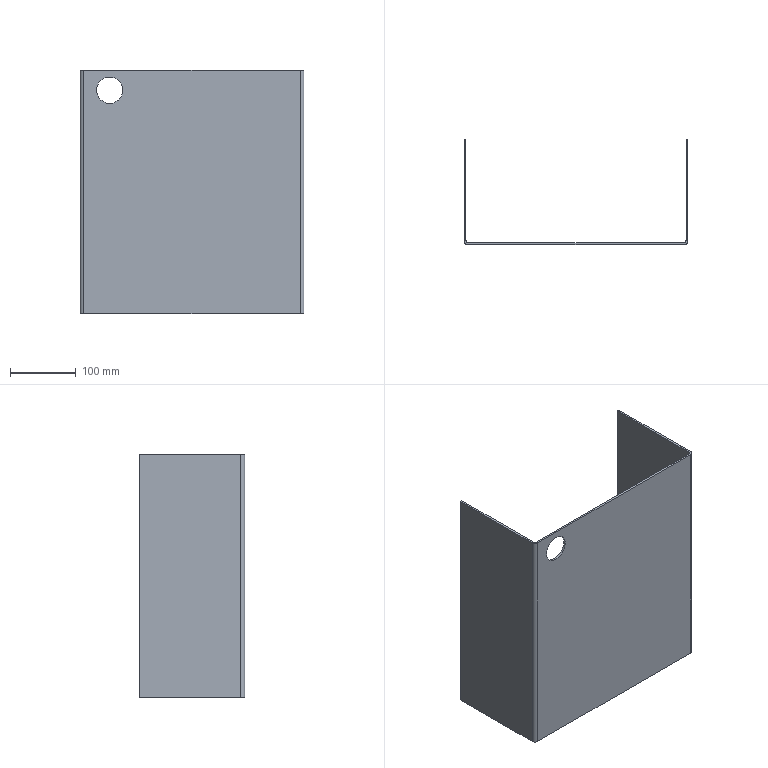Part | SolidWorks | features Cut 2, FlatPattern 1, SMBaseFlange 1, SheetMetal 1 | 1 solid | 26 faces | box 340 x 160 x 369 mm | volume 715620 mm3 | plane 18 | cylinder 8 | commonest cylinder face diameters 6 x2 11.5 x2 12 x2 40 x2
STEP:
#1=CARTESIAN_POINT('',(337.,145.,25.75));
#2=VERTEX_POINT('',#1);
#3=CARTESIAN_POINT('',(337.,145.,14.25));
#4=VERTEX_POINT('',#3);
#5=CARTESIAN_POINT('',(337.,145.,20.));
#6=DIRECTION('',(1.,0.,0.));
#7=DIRECTION('',(0.,0.,-1.));
#8=AXIS2_PLACEMENT_3D('',#5,#6,#7);
#9=CIRCLE('',#8,5.75);
#10=EDGE_CURVE('',#2,#4,#9,.T.);
#11=ORIENTED_EDGE('',*,*,#10,.F.);
#12=CARTESIAN_POINT('',(340.,145.,25.75));
#13=VERTEX_POINT('',#12);
#14=CARTESIAN_POINT('',(330.,145.,25.75));
#15=DIRECTION('',(1.,0.,0.));
#16=VECTOR('',#15,1000.);
#17=LINE('',#14,#16);
#18=EDGE_CURVE('',#2,#13,#17,.T.);
#19=ORIENTED_EDGE('',*,*,#18,.T.);
#20=CARTESIAN_POINT('',(340.,145.,14.25));
#21=VERTEX_POINT('',#20);
#22=CARTESIAN_POINT('',(340.,145.,20.));
#23=DIRECTION('',(1.,0.,0.));
#24=DIRECTION('',(0.,0.,-1.));
#25=AXIS2_PLACEMENT_3D('',#22,#23,#24);
#26=CIRCLE('',#25,5.75);
#27=EDGE_CURVE('',#13,#21,#26,.T.);
#28=ORIENTED_EDGE('',*,*,#27,.T.);
#29=CARTESIAN_POINT('',(330.,145.,14.25));
#30=DIRECTION('',(1.,0.,0.));
#31=VECTOR('',#30,1000.);
#32=LINE('',#29,#31);
#33=EDGE_CURVE('',#4,#21,#32,.T.);
#34=ORIENTED_EDGE('',*,*,#33,.F.);
#35=EDGE_LOOP('',(#11,#19,#28,#34));
#36=FACE_OUTER_BOUND('',#35,.T.);
#37=CARTESIAN_POINT('',(330.,145.,20.));
#38=DIRECTION('',(1.,0.,0.));
#39=DIRECTION('',(0.,0.,-1.));
#40=AXIS2_PLACEMENT_3D('',#37,#38,#39);
#41=CYLINDRICAL_SURFACE('',#40,5.75);
#42=ADVANCED_FACE('',(#36),#41,.F.);
#43=CARTESIAN_POINT('',(45.,3.,359.));
#44=VERTEX_POINT('',#43);
#45=CARTESIAN_POINT('',(45.,3.,319.));
#46=VERTEX_POINT('',#45);
#47=CARTESIAN_POINT('',(45.,3.,339.));
#48=DIRECTION('',(0.,-1.,0.));
#49=DIRECTION('',(0.,0.,-1.));
#50=AXIS2_PLACEMENT_3D('',#47,#48,#49);
#51=CIRCLE('',#50,20.);
#52=EDGE_CURVE('',#44,#46,#51,.T.);
#53=ORIENTED_EDGE('',*,*,#52,.F.);
#54=CARTESIAN_POINT('',(45.,0.,359.));
#55=VERTEX_POINT('',#54);
#56=CARTESIAN_POINT('',(45.,10.,359.));
#57=DIRECTION('',(0.,-1.,0.));
#58=VECTOR('',#57,1000.);
#59=LINE('',#56,#58);
#60=EDGE_CURVE('',#44,#55,#59,.T.);
#61=ORIENTED_EDGE('',*,*,#60,.T.);
#62=CARTESIAN_POINT('',(45.,0.,319.));
#63=VERTEX_POINT('',#62);
#64=CARTESIAN_POINT('',(45.,0.,339.));
#65=DIRECTION('',(0.,-1.,0.));
#66=DIRECTION('',(0.,0.,-1.));
#67=AXIS2_PLACEMENT_3D('',#64,#65,#66);
#68=CIRCLE('',#67,20.);
#69=EDGE_CURVE('',#55,#63,#68,.T.);
#70=ORIENTED_EDGE('',*,*,#69,.T.);
#71=CARTESIAN_POINT('',(45.,10.,319.));
#72=DIRECTION('',(0.,-1.,0.));
#73=VECTOR('',#72,1000.);
#74=LINE('',#71,#73);
#75=EDGE_CURVE('',#46,#63,#74,.T.);
#76=ORIENTED_EDGE('',*,*,#75,.F.);
#77=EDGE_LOOP('',(#53,#61,#70,#76));
#78=FACE_OUTER_BOUND('',#77,.T.);
#79=CARTESIAN_POINT('',(45.,10.,339.));
#80=DIRECTION('',(0.,-1.,0.));
#81=DIRECTION('',(0.,0.,-1.));
#82=AXIS2_PLACEMENT_3D('',#79,#80,#81);
#83=CYLINDRICAL_SURFACE('',#82,20.);
#84=ADVANCED_FACE('',(#78),#83,.F.);
#85=CARTESIAN_POINT('',(334.,0.,369.));
#86=VERTEX_POINT('',#85);
#87=CARTESIAN_POINT('',(334.,3.,369.));
#88=VERTEX_POINT('',#87);
#89=CARTESIAN_POINT('',(334.,0.,369.));
#90=DIRECTION('',(0.,1.,0.));
#91=VECTOR('',#90,1000.);
#92=LINE('',#89,#91);
#93=EDGE_CURVE('',#86,#88,#92,.T.);
#94=ORIENTED_EDGE('',*,*,#93,.F.);
#95=CARTESIAN_POINT('',(340.,6.,369.));
#96=VERTEX_POINT('',#95);
#97=CARTESIAN_POINT('',(334.,6.,369.));
#98=DIRECTION('',(0.,0.,-1.));
#99=DIRECTION('',(1.,0.,0.));
#100=AXIS2_PLACEMENT_3D('',#97,#98,#99);
#101=CIRCLE('',#100,6.);
#102=EDGE_CURVE('',#96,#86,#101,.T.);
#103=ORIENTED_EDGE('',*,*,#102,.F.);
#104=CARTESIAN_POINT('',(337.,6.,369.));
#105=VERTEX_POINT('',#104);
#106=CARTESIAN_POINT('',(337.,6.,369.));
#107=DIRECTION('',(1.,0.,0.));
#108=VECTOR('',#107,1000.);
#109=LINE('',#106,#108);
#110=EDGE_CURVE('',#105,#96,#109,.T.);
#111=ORIENTED_EDGE('',*,*,#110,.F.);
#112=CARTESIAN_POINT('',(334.,6.,369.));
#113=DIRECTION('',(0.,0.,-1.));
#114=DIRECTION('',(1.,0.,0.));
#115=AXIS2_PLACEMENT_3D('',#112,#113,#114);
#116=CIRCLE('',#115,3.);
#117=EDGE_CURVE('',#105,#88,#116,.T.);
#118=ORIENTED_EDGE('',*,*,#117,.T.);
#119=EDGE_LOOP('',(#94,#103,#111,#118));
#120=FACE_OUTER_BOUND('',#119,.T.);
#121=CARTESIAN_POINT('',(334.,0.,369.));
#122=DIRECTION('',(0.,0.,1.));
#123=DIRECTION('',(1.,0.,0.));
#124=AXIS2_PLACEMENT_3D('',#121,#122,#123);
#125=PLANE('',#124);
#126=ADVANCED_FACE('',(#120),#125,.T.);
#127=CARTESIAN_POINT('',(6.,0.,369.));
#128=VERTEX_POINT('',#127);
#129=CARTESIAN_POINT('',(0.,0.,369.));
#130=DIRECTION('',(-1.,0.,0.));
#131=VECTOR('',#130,1000.);
#132=LINE('',#129,#131);
#133=EDGE_CURVE('',#86,#128,#132,.T.);
#134=ORIENTED_EDGE('',*,*,#133,.F.);
#135=ORIENTED_EDGE('',*,*,#93,.T.);
#136=CARTESIAN_POINT('',(6.,3.,369.));
#137=VERTEX_POINT('',#136);
#138=CARTESIAN_POINT('',(0.,3.,369.));
#139=DIRECTION('',(-1.,0.,0.));
#140=VECTOR('',#139,1000.);
#141=LINE('',#138,#140);
#142=EDGE_CURVE('',#88,#137,#141,.T.);
#143=ORIENTED_EDGE('',*,*,#142,.T.);
#144=CARTESIAN_POINT('',(6.,3.,369.));
#145=DIRECTION('',(0.,-1.,0.));
#146=VECTOR('',#145,1000.);
#147=LINE('',#144,#146);
#148=EDGE_CURVE('',#137,#128,#147,.T.);
#149=ORIENTED_EDGE('',*,*,#148,.T.);
#150=EDGE_LOOP('',(#134,#135,#143,#149));
#151=FACE_OUTER_BOUND('',#150,.T.);
#152=CARTESIAN_POINT('',(337.,6.,369.));
#153=DIRECTION('',(0.,0.,1.));
#154=DIRECTION('',(1.,0.,0.));
#155=AXIS2_PLACEMENT_3D('',#152,#153,#154);
#156=PLANE('',#155);
#157=ADVANCED_FACE('',(#151),#156,.T.);
#158=CARTESIAN_POINT('',(340.,6.,0.));
#159=VERTEX_POINT('',#158);
#160=CARTESIAN_POINT('',(337.,6.,0.));
#161=VERTEX_POINT('',#160);
#162=CARTESIAN_POINT('',(340.,6.,0.));
#163=DIRECTION('',(-1.,0.,0.));
#164=VECTOR('',#163,1000.);
#165=LINE('',#162,#164);
#166=EDGE_CURVE('',#159,#161,#165,.T.);
#167=ORIENTED_EDGE('',*,*,#166,.F.);
#168=CARTESIAN_POINT('',(334.,0.,0.));
#169=VERTEX_POINT('',#168);
#170=CARTESIAN_POINT('',(334.,6.,0.));
#171=DIRECTION('',(0.,0.,-1.));
#172=DIRECTION('',(1.,0.,0.));
#173=AXIS2_PLACEMENT_3D('',#170,#171,#172);
#174=CIRCLE('',#173,6.);
#175=EDGE_CURVE('',#159,#169,#174,.T.);
#176=ORIENTED_EDGE('',*,*,#175,.T.);
#177=CARTESIAN_POINT('',(334.,3.,0.));
#178=VERTEX_POINT('',#177);
#179=CARTESIAN_POINT('',(334.,3.,0.));
#180=DIRECTION('',(0.,-1.,0.));
#181=VECTOR('',#180,1000.);
#182=LINE('',#179,#181);
#183=EDGE_CURVE('',#178,#169,#182,.T.);
#184=ORIENTED_EDGE('',*,*,#183,.F.);
#185=CARTESIAN_POINT('',(334.,6.,0.));
#186=DIRECTION('',(0.,0.,-1.));
#187=DIRECTION('',(1.,0.,0.));
#188=AXIS2_PLACEMENT_3D('',#185,#186,#187);
#189=CIRCLE('',#188,3.);
#190=EDGE_CURVE('',#161,#178,#189,.T.);
#191=ORIENTED_EDGE('',*,*,#190,.F.);
#192=EDGE_LOOP('',(#167,#176,#184,#191));
#193=FACE_OUTER_BOUND('',#192,.T.);
#194=CARTESIAN_POINT('',(340.,6.,0.));
#195=DIRECTION('',(0.,0.,-1.));
#196=DIRECTION('',(-1.,0.,0.));
#197=AXIS2_PLACEMENT_3D('',#194,#195,#196);
#198=PLANE('',#197);
#199=ADVANCED_FACE('',(#193),#198,.T.);
#200=CARTESIAN_POINT('',(340.,160.,0.));
#201=VERTEX_POINT('',#200);
#202=CARTESIAN_POINT('',(340.,0.,0.));
#203=DIRECTION('',(0.,-1.,0.));
#204=VECTOR('',#203,1000.);
#205=LINE('',#202,#204);
#206=EDGE_CURVE('',#201,#159,#205,.T.);
#207=ORIENTED_EDGE('',*,*,#206,.T.);
#208=ORIENTED_EDGE('',*,*,#166,.T.);
#209=CARTESIAN_POINT('',(337.,160.,0.));
#210=VERTEX_POINT('',#209);
#211=CARTESIAN_POINT('',(337.,0.,0.));
#212=DIRECTION('',(0.,-1.,0.));
#213=VECTOR('',#212,1000.);
#214=LINE('',#211,#213);
#215=EDGE_CURVE('',#210,#161,#214,.T.);
#216=ORIENTED_EDGE('',*,*,#215,.F.);
#217=CARTESIAN_POINT('',(337.,160.,0.));
#218=DIRECTION('',(1.,0.,0.));
#219=VECTOR('',#218,1000.);
#220=LINE('',#217,#219);
#221=EDGE_CURVE('',#210,#201,#220,.T.);
#222=ORIENTED_EDGE('',*,*,#221,.T.);
#223=EDGE_LOOP('',(#207,#208,#216,#222));
#224=FACE_OUTER_BOUND('',#223,.T.);
#225=CARTESIAN_POINT('',(334.,3.,0.));
#226=DIRECTION('',(0.,0.,-1.));
#227=DIRECTION('',(-1.,0.,0.));
#228=AXIS2_PLACEMENT_3D('',#225,#226,#227);
#229=PLANE('',#228);
#230=ADVANCED_FACE('',(#224),#229,.T.);
#231=CARTESIAN_POINT('',(0.,6.,369.));
#232=VERTEX_POINT('',#231);
#233=CARTESIAN_POINT('',(3.,6.,369.));
#234=VERTEX_POINT('',#233);
#235=CARTESIAN_POINT('',(0.,6.,369.));
#236=DIRECTION('',(1.,0.,0.));
#237=VECTOR('',#236,1000.);
#238=LINE('',#235,#237);
#239=EDGE_CURVE('',#232,#234,#238,.T.);
#240=ORIENTED_EDGE('',*,*,#239,.F.);
#241=CARTESIAN_POINT('',(6.,6.,369.));
#242=DIRECTION('',(0.,0.,-1.));
#243=DIRECTION('',(1.,0.,0.));
#244=AXIS2_PLACEMENT_3D('',#241,#242,#243);
#245=CIRCLE('',#244,6.);
#246=EDGE_CURVE('',#128,#232,#245,.T.);
#247=ORIENTED_EDGE('',*,*,#246,.F.);
#248=ORIENTED_EDGE('',*,*,#148,.F.);
#249=CARTESIAN_POINT('',(6.,6.,369.));
#250=DIRECTION('',(0.,0.,-1.));
#251=DIRECTION('',(1.,0.,0.));
#252=AXIS2_PLACEMENT_3D('',#249,#250,#251);
#253=CIRCLE('',#252,3.);
#254=EDGE_CURVE('',#137,#234,#253,.T.);
#255=ORIENTED_EDGE('',*,*,#254,.T.);
#256=EDGE_LOOP('',(#240,#247,#248,#255));
#257=FACE_OUTER_BOUND('',#256,.T.);
#258=CARTESIAN_POINT('',(0.,6.,369.));
#259=DIRECTION('',(0.,0.,1.));
#260=DIRECTION('',(1.,0.,0.));
#261=AXIS2_PLACEMENT_3D('',#258,#259,#260);
#262=PLANE('',#261);
#263=ADVANCED_FACE('',(#257),#262,.T.);
#264=CARTESIAN_POINT('',(0.,160.,369.));
#265=VERTEX_POINT('',#264);
#266=CARTESIAN_POINT('',(0.,0.,369.));
#267=DIRECTION('',(0.,1.,0.));
#268=VECTOR('',#267,1000.);
#269=LINE('',#266,#268);
#270=EDGE_CURVE('',#232,#265,#269,.T.);
#271=ORIENTED_EDGE('',*,*,#270,.F.);
#272=ORIENTED_EDGE('',*,*,#239,.T.);
#273=CARTESIAN_POINT('',(3.,160.,369.));
#274=VERTEX_POINT('',#273);
#275=CARTESIAN_POINT('',(3.,0.,369.));
#276=DIRECTION('',(0.,1.,0.));
#277=VECTOR('',#276,1000.);
#278=LINE('',#275,#277);
#279=EDGE_CURVE('',#234,#274,#278,.T.);
#280=ORIENTED_EDGE('',*,*,#279,.T.);
#281=CARTESIAN_POINT('',(0.,160.,369.));
#282=DIRECTION('',(1.,0.,0.));
#283=VECTOR('',#282,1000.);
#284=LINE('',#281,#283);
#285=EDGE_CURVE('',#265,#274,#284,.T.);
#286=ORIENTED_EDGE('',*,*,#285,.F.);
#287=EDGE_LOOP('',(#271,#272,#280,#286));
#288=FACE_OUTER_BOUND('',#287,.T.);
#289=CARTESIAN_POINT('',(6.,3.,369.));
#290=DIRECTION('',(0.,0.,1.));
#291=DIRECTION('',(1.,0.,0.));
#292=AXIS2_PLACEMENT_3D('',#289,#290,#291);
#293=PLANE('',#292);
#294=ADVANCED_FACE('',(#288),#293,.T.);
#295=CARTESIAN_POINT('',(6.,0.,0.));
#296=VERTEX_POINT('',#295);
#297=CARTESIAN_POINT('',(6.,3.,0.));
#298=VERTEX_POINT('',#297);
#299=CARTESIAN_POINT('',(6.,0.,0.));
#300=DIRECTION('',(0.,1.,0.));
#301=VECTOR('',#300,1000.);
#302=LINE('',#299,#301);
#303=EDGE_CURVE('',#296,#298,#302,.T.);
#304=ORIENTED_EDGE('',*,*,#303,.F.);
#305=CARTESIAN_POINT('',(0.,6.,0.));
#306=VERTEX_POINT('',#305);
#307=CARTESIAN_POINT('',(6.,6.,0.));
#308=DIRECTION('',(0.,0.,-1.));
#309=DIRECTION('',(1.,0.,0.));
#310=AXIS2_PLACEMENT_3D('',#307,#308,#309);
#311=CIRCLE('',#310,6.);
#312=EDGE_CURVE('',#296,#306,#311,.T.);
#313=ORIENTED_EDGE('',*,*,#312,.T.);
#314=CARTESIAN_POINT('',(3.,6.,0.));
#315=VERTEX_POINT('',#314);
#316=CARTESIAN_POINT('',(3.,6.,0.));
#317=DIRECTION('',(-1.,0.,0.));
#318=VECTOR('',#317,1000.);
#319=LINE('',#316,#318);
#320=EDGE_CURVE('',#315,#306,#319,.T.);
#321=ORIENTED_EDGE('',*,*,#320,.F.);
#322=CARTESIAN_POINT('',(6.,6.,0.));
#323=DIRECTION('',(0.,0.,-1.));
#324=DIRECTION('',(1.,0.,0.));
#325=AXIS2_PLACEMENT_3D('',#322,#323,#324);
#326=CIRCLE('',#325,3.);
#327=EDGE_CURVE('',#298,#315,#326,.T.);
#328=ORIENTED_EDGE('',*,*,#327,.F.);
#329=EDGE_LOOP('',(#304,#313,#321,#328));
#330=FACE_OUTER_BOUND('',#329,.T.);
#331=CARTESIAN_POINT('',(6.,0.,0.));
#332=DIRECTION('',(0.,0.,-1.));
#333=DIRECTION('',(-1.,0.,0.));
#334=AXIS2_PLACEMENT_3D('',#331,#332,#333);
#335=PLANE('',#334);
#336=ADVANCED_FACE('',(#330),#335,.T.);
#337=CARTESIAN_POINT('',(0.,0.,0.));
#338=DIRECTION('',(-1.,0.,0.));
#339=VECTOR('',#338,1000.);
#340=LINE('',#337,#339);
#341=EDGE_CURVE('',#169,#296,#340,.T.);
#342=ORIENTED_EDGE('',*,*,#341,.T.);
#343=ORIENTED_EDGE('',*,*,#303,.T.);
#344=CARTESIAN_POINT('',(0.,3.,0.));
#345=DIRECTION('',(-1.,0.,0.));
#346=VECTOR('',#345,1000.);
#347=LINE('',#344,#346);
#348=EDGE_CURVE('',#178,#298,#347,.T.);
#349=ORIENTED_EDGE('',*,*,#348,.F.);
#350=ORIENTED_EDGE('',*,*,#183,.T.);
#351=EDGE_LOOP('',(#342,#343,#349,#350));
#352=FACE_OUTER_BOUND('',#351,.T.);
#353=CARTESIAN_POINT('',(3.,6.,0.));
#354=DIRECTION('',(0.,0.,-1.));
#355=DIRECTION('',(-1.,0.,0.));
#356=AXIS2_PLACEMENT_3D('',#353,#354,#355);
#357=PLANE('',#356);
#358=ADVANCED_FACE('',(#352),#357,.T.);
#359=CARTESIAN_POINT('',(3.,160.,0.));
#360=VERTEX_POINT('',#359);
#361=CARTESIAN_POINT('',(3.,0.,0.));
#362=DIRECTION('',(0.,1.,0.));
#363=VECTOR('',#362,1000.);
#364=LINE('',#361,#363);
#365=EDGE_CURVE('',#315,#360,#364,.T.);
#366=ORIENTED_EDGE('',*,*,#365,.T.);
#367=CARTESIAN_POINT('',(3.,160.,369.));
#368=DIRECTION('',(0.,0.,-1.));
#369=VECTOR('',#368,1000.);
#370=LINE('',#367,#369);
#371=EDGE_CURVE('',#274,#360,#370,.T.);
#372=ORIENTED_EDGE('',*,*,#371,.F.);
#373=ORIENTED_EDGE('',*,*,#279,.F.);
#374=CARTESIAN_POINT('',(3.,6.,369.));
#375=DIRECTION('',(0.,0.,-1.));
#376=VECTOR('',#375,1000.);
#377=LINE('',#374,#376);
#378=EDGE_CURVE('',#234,#315,#377,.T.);
#379=ORIENTED_EDGE('',*,*,#378,.T.);
#380=EDGE_LOOP('',(#366,#372,#373,#379));
#381=FACE_OUTER_BOUND('',#380,.T.);
#382=CARTESIAN_POINT('',(3.,0.,369.));
#383=DIRECTION('',(-1.,0.,0.));
#384=DIRECTION('',(0.,0.,1.));
#385=AXIS2_PLACEMENT_3D('',#382,#383,#384);
#386=PLANE('',#385);
#387=ADVANCED_FACE('',(#381),#386,.F.);
#388=CARTESIAN_POINT('',(0.,160.,0.));
#389=VERTEX_POINT('',#388);
#390=CARTESIAN_POINT('',(0.,160.,0.));
#391=DIRECTION('',(1.,0.,0.));
#392=VECTOR('',#391,1000.);
#393=LINE('',#390,#392);
#394=EDGE_CURVE('',#389,#360,#393,.T.);
#395=ORIENTED_EDGE('',*,*,#394,.F.);
#396=CARTESIAN_POINT('',(0.,160.,369.));
#397=DIRECTION('',(0.,0.,-1.));
#398=VECTOR('',#397,1000.);
#399=LINE('',#396,#398);
#400=EDGE_CURVE('',#265,#389,#399,.T.);
#401=ORIENTED_EDGE('',*,*,#400,.F.);
#402=ORIENTED_EDGE('',*,*,#285,.T.);
#403=ORIENTED_EDGE('',*,*,#371,.T.);
#404=EDGE_LOOP('',(#395,#401,#402,#403));
#405=FACE_OUTER_BOUND('',#404,.T.);
#406=CARTESIAN_POINT('',(0.,160.,369.));
#407=DIRECTION('',(0.,1.,0.));
#408=DIRECTION('',(0.,0.,1.));
#409=AXIS2_PLACEMENT_3D('',#406,#407,#408);
#410=PLANE('',#409);
#411=ADVANCED_FACE('',(#405),#410,.T.);
#412=CARTESIAN_POINT('',(0.,0.,0.));
#413=DIRECTION('',(0.,1.,0.));
#414=VECTOR('',#413,1000.);
#415=LINE('',#412,#414);
#416=EDGE_CURVE('',#306,#389,#415,.T.);
#417=ORIENTED_EDGE('',*,*,#416,.F.);
#418=CARTESIAN_POINT('',(0.,6.,369.));
#419=DIRECTION('',(0.,0.,-1.));
#420=VECTOR('',#419,1000.);
#421=LINE('',#418,#420);
#422=EDGE_CURVE('',#232,#306,#421,.T.);
#423=ORIENTED_EDGE('',*,*,#422,.F.);
#424=ORIENTED_EDGE('',*,*,#270,.T.);
#425=ORIENTED_EDGE('',*,*,#400,.T.);
#426=EDGE_LOOP('',(#417,#423,#424,#425));
#427=FACE_OUTER_BOUND('',#426,.T.);
#428=CARTESIAN_POINT('',(0.,0.,369.));
#429=DIRECTION('',(-1.,0.,0.));
#430=DIRECTION('',(0.,0.,1.));
#431=AXIS2_PLACEMENT_3D('',#428,#429,#430);
#432=PLANE('',#431);
#433=ADVANCED_FACE('',(#427),#432,.T.);
#434=ORIENTED_EDGE('',*,*,#312,.F.);
#435=CARTESIAN_POINT('',(6.,0.,369.));
#436=DIRECTION('',(0.,0.,-1.));
#437=VECTOR('',#436,1000.);
#438=LINE('',#435,#437);
#439=EDGE_CURVE('',#128,#296,#438,.T.);
#440=ORIENTED_EDGE('',*,*,#439,.F.);
#441=ORIENTED_EDGE('',*,*,#246,.T.);
#442=ORIENTED_EDGE('',*,*,#422,.T.);
#443=EDGE_LOOP('',(#434,#440,#441,#442));
#444=FACE_OUTER_BOUND('',#443,.T.);
#445=CARTESIAN_POINT('',(6.,6.,369.));
#446=DIRECTION('',(0.,0.,-1.));
#447=DIRECTION('',(-1.,0.,0.));
#448=AXIS2_PLACEMENT_3D('',#445,#446,#447);
#449=CYLINDRICAL_SURFACE('',#448,6.);
#450=ADVANCED_FACE('',(#444),#449,.T.);
#451=CARTESIAN_POINT('',(45.,0.,339.));
#452=DIRECTION('',(0.,-1.,0.));
#453=DIRECTION('',(0.,0.,-1.));
#454=AXIS2_PLACEMENT_3D('',#451,#452,#453);
#455=CIRCLE('',#454,20.);
#456=EDGE_CURVE('',#63,#55,#455,.T.);
#457=ORIENTED_EDGE('',*,*,#456,.F.);
#458=ORIENTED_EDGE('',*,*,#69,.F.);
#459=EDGE_LOOP('',(#457,#458));
#460=FACE_BOUND('',#459,.T.);
#461=ORIENTED_EDGE('',*,*,#341,.F.);
#462=CARTESIAN_POINT('',(334.,0.,369.));
#463=DIRECTION('',(0.,0.,-1.));
#464=VECTOR('',#463,1000.);
#465=LINE('',#462,#464);
#466=EDGE_CURVE('',#86,#169,#465,.T.);
#467=ORIENTED_EDGE('',*,*,#466,.F.);
#468=ORIENTED_EDGE('',*,*,#133,.T.);
#469=ORIENTED_EDGE('',*,*,#439,.T.);
#470=EDGE_LOOP('',(#461,#467,#468,#469));
#471=FACE_OUTER_BOUND('',#470,.T.);
#472=CARTESIAN_POINT('',(0.,0.,369.));
#473=DIRECTION('',(0.,-1.,0.));
#474=DIRECTION('',(0.,0.,-1.));
#475=AXIS2_PLACEMENT_3D('',#472,#473,#474);
#476=PLANE('',#475);
#477=ADVANCED_FACE('',(#460,#471),#476,.T.);
#478=ORIENTED_EDGE('',*,*,#175,.F.);
#479=CARTESIAN_POINT('',(340.,6.,369.));
#480=DIRECTION('',(0.,0.,-1.));
#481=VECTOR('',#480,1000.);
#482=LINE('',#479,#481);
#483=EDGE_CURVE('',#96,#159,#482,.T.);
#484=ORIENTED_EDGE('',*,*,#483,.F.);
#485=ORIENTED_EDGE('',*,*,#102,.T.);
#486=ORIENTED_EDGE('',*,*,#466,.T.);
#487=EDGE_LOOP('',(#478,#484,#485,#486));
#488=FACE_OUTER_BOUND('',#487,.T.);
#489=CARTESIAN_POINT('',(334.,6.,369.));
#490=DIRECTION('',(0.,0.,-1.));
#491=DIRECTION('',(-1.,0.,0.));
#492=AXIS2_PLACEMENT_3D('',#489,#490,#491);
#493=CYLINDRICAL_SURFACE('',#492,6.);
#494=ADVANCED_FACE('',(#488),#493,.T.);
#495=CARTESIAN_POINT('',(340.,145.,20.));
#496=DIRECTION('',(1.,0.,0.));
#497=DIRECTION('',(0.,0.,-1.));
#498=AXIS2_PLACEMENT_3D('',#495,#496,#497);
#499=CIRCLE('',#498,5.75);
#500=EDGE_CURVE('',#21,#13,#499,.T.);
#501=ORIENTED_EDGE('',*,*,#500,.F.);
#502=ORIENTED_EDGE('',*,*,#27,.F.);
#503=EDGE_LOOP('',(#501,#502));
#504=FACE_BOUND('',#503,.T.);
#505=ORIENTED_EDGE('',*,*,#206,.F.);
#506=CARTESIAN_POINT('',(340.,160.,369.));
#507=VERTEX_POINT('',#506);
#508=CARTESIAN_POINT('',(340.,160.,369.));
#509=DIRECTION('',(0.,0.,-1.));
#510=VECTOR('',#509,1000.);
#511=LINE('',#508,#510);
#512=EDGE_CURVE('',#507,#201,#511,.T.);
#513=ORIENTED_EDGE('',*,*,#512,.F.);
#514=CARTESIAN_POINT('',(340.,0.,369.));
#515=DIRECTION('',(0.,-1.,0.));
#516=VECTOR('',#515,1000.);
#517=LINE('',#514,#516);
#518=EDGE_CURVE('',#507,#96,#517,.T.);
#519=ORIENTED_EDGE('',*,*,#518,.T.);
#520=ORIENTED_EDGE('',*,*,#483,.T.);
#521=EDGE_LOOP('',(#505,#513,#519,#520));
#522=FACE_OUTER_BOUND('',#521,.T.);
#523=CARTESIAN_POINT('',(340.,0.,369.));
#524=DIRECTION('',(1.,0.,0.));
#525=DIRECTION('',(0.,0.,-1.));
#526=AXIS2_PLACEMENT_3D('',#523,#524,#525);
#527=PLANE('',#526);
#528=ADVANCED_FACE('',(#504,#522),#527,.T.);
#529=ORIENTED_EDGE('',*,*,#221,.F.);
#530=CARTESIAN_POINT('',(337.,160.,369.));
#531=VERTEX_POINT('',#530);
#532=CARTESIAN_POINT('',(337.,160.,369.));
#533=DIRECTION('',(0.,0.,-1.));
#534=VECTOR('',#533,1000.);
#535=LINE('',#532,#534);
#536=EDGE_CURVE('',#531,#210,#535,.T.);
#537=ORIENTED_EDGE('',*,*,#536,.F.);
#538=CARTESIAN_POINT('',(337.,160.,369.));
#539=DIRECTION('',(1.,0.,0.));
#540=VECTOR('',#539,1000.);
#541=LINE('',#538,#540);
#542=EDGE_CURVE('',#531,#507,#541,.T.);
#543=ORIENTED_EDGE('',*,*,#542,.T.);
#544=ORIENTED_EDGE('',*,*,#512,.T.);
#545=EDGE_LOOP('',(#529,#537,#543,#544));
#546=FACE_OUTER_BOUND('',#545,.T.);
#547=CARTESIAN_POINT('',(337.,160.,369.));
#548=DIRECTION('',(0.,1.,0.));
#549=DIRECTION('',(0.,0.,1.));
#550=AXIS2_PLACEMENT_3D('',#547,#548,#549);
#551=PLANE('',#550);
#552=ADVANCED_FACE('',(#546),#551,.T.);
#553=CARTESIAN_POINT('',(337.,145.,20.));
#554=DIRECTION('',(1.,0.,0.));
#555=DIRECTION('',(0.,0.,-1.));
#556=AXIS2_PLACEMENT_3D('',#553,#554,#555);
#557=CIRCLE('',#556,5.75);
#558=EDGE_CURVE('',#4,#2,#557,.T.);
#559=ORIENTED_EDGE('',*,*,#558,.T.);
#560=ORIENTED_EDGE('',*,*,#10,.T.);
#561=EDGE_LOOP('',(#559,#560));
#562=FACE_BOUND('',#561,.T.);
#563=ORIENTED_EDGE('',*,*,#215,.T.);
#564=CARTESIAN_POINT('',(337.,6.,369.));
#565=DIRECTION('',(0.,0.,-1.));
#566=VECTOR('',#565,1000.);
#567=LINE('',#564,#566);
#568=EDGE_CURVE('',#105,#161,#567,.T.);
#569=ORIENTED_EDGE('',*,*,#568,.F.);
#570=CARTESIAN_POINT('',(337.,0.,369.));
#571=DIRECTION('',(0.,-1.,0.));
#572=VECTOR('',#571,1000.);
#573=LINE('',#570,#572);
#574=EDGE_CURVE('',#531,#105,#573,.T.);
#575=ORIENTED_EDGE('',*,*,#574,.F.);
#576=ORIENTED_EDGE('',*,*,#536,.T.);
#577=EDGE_LOOP('',(#563,#569,#575,#576));
#578=FACE_OUTER_BOUND('',#577,.T.);
#579=CARTESIAN_POINT('',(337.,0.,369.));
#580=DIRECTION('',(1.,0.,0.));
#581=DIRECTION('',(0.,0.,-1.));
#582=AXIS2_PLACEMENT_3D('',#579,#580,#581);
#583=PLANE('',#582);
#584=ADVANCED_FACE('',(#562,#578),#583,.F.);
#585=ORIENTED_EDGE('',*,*,#190,.T.);
#586=CARTESIAN_POINT('',(334.,3.,369.));
#587=DIRECTION('',(0.,0.,-1.));
#588=VECTOR('',#587,1000.);
#589=LINE('',#586,#588);
#590=EDGE_CURVE('',#88,#178,#589,.T.);
#591=ORIENTED_EDGE('',*,*,#590,.F.);
#592=ORIENTED_EDGE('',*,*,#117,.F.);
#593=ORIENTED_EDGE('',*,*,#568,.T.);
#594=EDGE_LOOP('',(#585,#591,#592,#593));
#595=FACE_OUTER_BOUND('',#594,.T.);
#596=CARTESIAN_POINT('',(334.,6.,369.));
#597=DIRECTION('',(0.,0.,-1.));
#598=DIRECTION('',(-1.,0.,0.));
#599=AXIS2_PLACEMENT_3D('',#596,#597,#598);
#600=CYLINDRICAL_SURFACE('',#599,3.);
#601=ADVANCED_FACE('',(#595),#600,.F.);
#602=CARTESIAN_POINT('',(45.,3.,339.));
#603=DIRECTION('',(0.,-1.,0.));
#604=DIRECTION('',(0.,0.,-1.));
#605=AXIS2_PLACEMENT_3D('',#602,#603,#604);
#606=CIRCLE('',#605,20.);
#607=EDGE_CURVE('',#46,#44,#606,.T.);
#608=ORIENTED_EDGE('',*,*,#607,.T.);
#609=ORIENTED_EDGE('',*,*,#52,.T.);
#610=EDGE_LOOP('',(#608,#609));
#611=FACE_BOUND('',#610,.T.);
#612=ORIENTED_EDGE('',*,*,#348,.T.);
#613=CARTESIAN_POINT('',(6.,3.,369.));
#614=DIRECTION('',(0.,0.,-1.));
#615=VECTOR('',#614,1000.);
#616=LINE('',#613,#615);
#617=EDGE_CURVE('',#137,#298,#616,.T.);
#618=ORIENTED_EDGE('',*,*,#617,.F.);
#619=ORIENTED_EDGE('',*,*,#142,.F.);
#620=ORIENTED_EDGE('',*,*,#590,.T.);
#621=EDGE_LOOP('',(#612,#618,#619,#620));
#622=FACE_OUTER_BOUND('',#621,.T.);
#623=CARTESIAN_POINT('',(0.,3.,369.));
#624=DIRECTION('',(0.,-1.,0.));
#625=DIRECTION('',(0.,0.,-1.));
#626=AXIS2_PLACEMENT_3D('',#623,#624,#625);
#627=PLANE('',#626);
#628=ADVANCED_FACE('',(#611,#622),#627,.F.);
#629=ORIENTED_EDGE('',*,*,#327,.T.);
#630=ORIENTED_EDGE('',*,*,#378,.F.);
#631=ORIENTED_EDGE('',*,*,#254,.F.);
#632=ORIENTED_EDGE('',*,*,#617,.T.);
#633=EDGE_LOOP('',(#629,#630,#631,#632));
#634=FACE_OUTER_BOUND('',#633,.T.);
#635=CARTESIAN_POINT('',(6.,6.,369.));
#636=DIRECTION('',(0.,0.,-1.));
#637=DIRECTION('',(-1.,0.,0.));
#638=AXIS2_PLACEMENT_3D('',#635,#636,#637);
#639=CYLINDRICAL_SURFACE('',#638,3.);
#640=ADVANCED_FACE('',(#634),#639,.F.);
#641=ORIENTED_EDGE('',*,*,#574,.T.);
#642=ORIENTED_EDGE('',*,*,#110,.T.);
#643=ORIENTED_EDGE('',*,*,#518,.F.);
#644=ORIENTED_EDGE('',*,*,#542,.F.);
#645=EDGE_LOOP('',(#641,#642,#643,#644));
#646=FACE_OUTER_BOUND('',#645,.T.);
#647=CARTESIAN_POINT('',(6.,6.,369.));
#648=DIRECTION('',(0.,0.,1.));
#649=DIRECTION('',(1.,0.,0.));
#650=AXIS2_PLACEMENT_3D('',#647,#648,#649);
#651=PLANE('',#650);
#652=ADVANCED_FACE('',(#646),#651,.T.);
#653=ORIENTED_EDGE('',*,*,#365,.F.);
#654=ORIENTED_EDGE('',*,*,#320,.T.);
#655=ORIENTED_EDGE('',*,*,#416,.T.);
#656=ORIENTED_EDGE('',*,*,#394,.T.);
#657=EDGE_LOOP('',(#653,#654,#655,#656));
#658=FACE_OUTER_BOUND('',#657,.T.);
#659=CARTESIAN_POINT('',(6.,6.,0.));
#660=DIRECTION('',(0.,0.,1.));
#661=DIRECTION('',(1.,0.,0.));
#662=AXIS2_PLACEMENT_3D('',#659,#660,#661);
#663=PLANE('',#662);
#664=ADVANCED_FACE('',(#658),#663,.F.);
#665=ORIENTED_EDGE('',*,*,#60,.F.);
#666=ORIENTED_EDGE('',*,*,#607,.F.);
#667=ORIENTED_EDGE('',*,*,#75,.T.);
#668=ORIENTED_EDGE('',*,*,#456,.T.);
#669=EDGE_LOOP('',(#665,#666,#667,#668));
#670=FACE_OUTER_BOUND('',#669,.T.);
#671=CARTESIAN_POINT('',(45.,10.,339.));
#672=DIRECTION('',(0.,-1.,0.));
#673=DIRECTION('',(0.,0.,-1.));
#674=AXIS2_PLACEMENT_3D('',#671,#672,#673);
#675=CYLINDRICAL_SURFACE('',#674,20.);
#676=ADVANCED_FACE('',(#670),#675,.F.);
#677=ORIENTED_EDGE('',*,*,#18,.F.);
#678=ORIENTED_EDGE('',*,*,#558,.F.);
#679=ORIENTED_EDGE('',*,*,#33,.T.);
#680=ORIENTED_EDGE('',*,*,#500,.T.);
#681=EDGE_LOOP('',(#677,#678,#679,#680));
#682=FACE_OUTER_BOUND('',#681,.T.);
#683=CARTESIAN_POINT('',(330.,145.,20.));
#684=DIRECTION('',(1.,0.,0.));
#685=DIRECTION('',(0.,0.,-1.));
#686=AXIS2_PLACEMENT_3D('',#683,#684,#685);
#687=CYLINDRICAL_SURFACE('',#686,5.75);
#688=ADVANCED_FACE('',(#682),#687,.F.);
#689=CLOSED_SHELL('',(#42,#84,#126,#157,#199,#230,#263,#294,#336,#358,#387,#411,#433,#450,#477,#494,#528,#552,#584,#601,#628,#640,#652,#664,#676,#688));
#690=MANIFOLD_SOLID_BREP('',#689);
#691=CARTESIAN_POINT('',(0.,0.,0.));
#692=DIRECTION('',(0.,0.,1.));
#693=DIRECTION('',(1.,0.,0.));
#694=AXIS2_PLACEMENT_3D('',#691,#692,#693);
#695=(LENGTH_UNIT()NAMED_UNIT(*)SI_UNIT(.MILLI.,.METRE.));
#696=UNCERTAINTY_MEASURE_WITH_UNIT(LENGTH_MEASURE(0.00001),#695,'','');
#697=(NAMED_UNIT(*)PLANE_ANGLE_UNIT()SI_UNIT($,.RADIAN.));
#698=(NAMED_UNIT(*)SI_UNIT($,.STERADIAN.)SOLID_ANGLE_UNIT());
#699=(GEOMETRIC_REPRESENTATION_CONTEXT(3)GLOBAL_UNCERTAINTY_ASSIGNED_CONTEXT((#696))GLOBAL_UNIT_ASSIGNED_CONTEXT((#695,#697,#698))REPRESENTATION_CONTEXT('',''));
#700=ADVANCED_BREP_SHAPE_REPRESENTATION('',(#690,#694),#699);